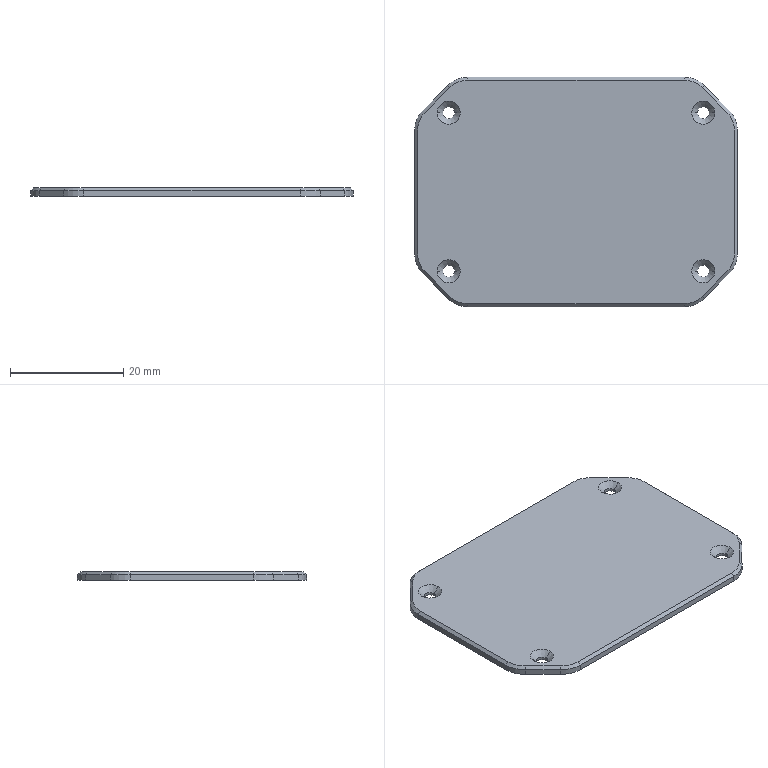NC program | NX | posted with a generic post | part box 57 x 40.5 x 1.5 mm
Lines 4444 to 5919 of 7802:
(PLANAR_PROFILE_COPY_2_COPY_1 , TOOL : D4)
N8676 T01 M6
N8678 G54
N8680 G17 G0 G90 X-121.9 Y151.609 S6500 M3
N8682 G43 Z20. H1
N8684 Z0.1
N8686 G94 G1 Y128.668 Z0.06 F1200.
N8688 X-122.173 Y127.266 Z0.057
N8690 X-122.719 Y125.947 Z0.055
N8692 X-123.518 Y124.763 Z0.052
N8694 X-128.763 Y119.518 Z0.04
N8696 X-129.947 Y118.719 Z0.037
N8698 X-131.266 Y118.173 Z0.035
N8700 X-132.668 Y117.9 Z0.032
N8702 X-172.332 Z-0.037
N8704 X-173.734 Y118.173 Z-0.04
N8706 X-175.053 Y118.719 Z-0.042
N8708 X-176.237 Y119.518 Z-0.045
N8710 X-181.482 Y124.763 Z-0.058
N8712 X-182.281 Y125.947 Z-0.06
N8714 X-182.827 Y127.266 Z-0.063
N8716 X-183.1 Y128.668 Z-0.065
N8718 Y151.832 Z-0.106
N8720 X-182.827 Y153.234 Z-0.108
N8722 X-182.281 Y154.553 Z-0.11
N8724 X-181.482 Y155.737 Z-0.113
N8726 X-176.237 Y160.982 Z-0.126
N8728 X-175.053 Y161.781 Z-0.128
N8730 X-173.734 Y162.327 Z-0.131
N8732 X-172.332 Y162.6 Z-0.133
N8734 X-132.668 Z-0.203
N8736 X-131.266 Y162.327 Z-0.205
N8738 X-129.947 Y161.781 Z-0.208
N8740 X-128.763 Y160.982 Z-0.21
N8742 X-123.518 Y155.737 Z-0.223
N8744 X-122.719 Y154.553 Z-0.226
N8746 X-122.173 Y153.234 Z-0.228
N8748 X-121.9 Y151.832 Z-0.231
N8750 Y128.668 Z-0.271
N8752 X-122.173 Y127.266 Z-0.273
N8754 X-122.719 Y125.947 Z-0.276
N8756 X-123.518 Y124.763 Z-0.278
N8758 X-128.763 Y119.518 Z-0.291
N8760 X-129.947 Y118.719 Z-0.294
N8762 X-131.266 Y118.173 Z-0.296
N8764 X-132.668 Y117.9 Z-0.299
N8766 X-133.321 Z-0.3
N8768 X-171.679 F2000.
N8770 G2 X-176.699 Y119.98 R7.1
N8772 G1 X-181.02 Y124.301
N8774 G2 X-183.1 Y129.321 R7.1
N8776 G1 Y151.179
N8778 G2 X-181.02 Y156.199 R7.1
N8780 G1 X-176.699 Y160.52
N8782 G2 X-171.679 Y162.6 R7.1
N8784 G1 X-133.321
N8786 G2 X-128.301 Y160.52 R7.1
N8788 G1 X-123.98 Y156.199
N8790 G2 X-121.9 Y151.179 R7.1
N8792 G1 Y129.321
N8794 G2 X-123.98 Y124.301 R7.1
N8796 G1 X-128.301 Y119.98
N8798 G2 X-133.321 Y117.9 R7.1
N8800 G1 Z-0.2
N8802 G0 Z20.
N8804 X-121.9 Y151.609
N8806 Z-0.2
N8808 G1 Y128.668 Z-0.24 F1200.
N8810 X-122.173 Y127.266 Z-0.243
N8812 X-122.719 Y125.947 Z-0.245
N8814 X-123.518 Y124.763 Z-0.248
N8816 X-128.763 Y119.518 Z-0.26
N8818 X-129.947 Y118.719 Z-0.263
N8820 X-131.266 Y118.173 Z-0.265
N8822 X-132.668 Y117.9 Z-0.268
N8824 X-172.332 Z-0.337
N8826 X-173.734 Y118.173 Z-0.34
N8828 X-175.053 Y118.719 Z-0.342
N8830 X-176.237 Y119.518 Z-0.345
N8832 X-181.482 Y124.763 Z-0.358
N8834 X-182.281 Y125.947 Z-0.36
N8836 X-182.827 Y127.266 Z-0.363
N8838 X-183.1 Y128.668 Z-0.365
N8840 Y151.832 Z-0.406
N8842 X-182.827 Y153.234 Z-0.408
N8844 X-182.281 Y154.553 Z-0.41
N8846 X-181.482 Y155.737 Z-0.413
N8848 X-176.237 Y160.982 Z-0.426
N8850 X-175.053 Y161.781 Z-0.428
N8852 X-173.734 Y162.327 Z-0.431
N8854 X-172.332 Y162.6 Z-0.433
N8856 X-132.668 Z-0.503
N8858 X-131.266 Y162.327 Z-0.505
N8860 X-129.947 Y161.781 Z-0.508
N8862 X-128.763 Y160.982 Z-0.51
N8864 X-123.518 Y155.737 Z-0.523
N8866 X-122.719 Y154.553 Z-0.526
N8868 X-122.173 Y153.234 Z-0.528
N8870 X-121.9 Y151.832 Z-0.531
N8872 Y128.668 Z-0.571
N8874 X-122.173 Y127.266 Z-0.573
N8876 X-122.719 Y125.947 Z-0.576
N8878 X-123.518 Y124.763 Z-0.578
N8880 X-128.763 Y119.518 Z-0.591
N8882 X-129.947 Y118.719 Z-0.594
N8884 X-131.266 Y118.173 Z-0.596
N8886 X-132.668 Y117.9 Z-0.599
N8888 X-133.321 Z-0.6
N8890 X-171.679 F2000.
N8892 G2 X-176.699 Y119.98 R7.1
N8894 G1 X-181.02 Y124.301
N8896 G2 X-183.1 Y129.321 R7.1
N8898 G1 Y151.179
N8900 G2 X-181.02 Y156.199 R7.1
N8902 G1 X-176.699 Y160.52
N8904 G2 X-171.679 Y162.6 R7.1
N8906 G1 X-133.321
N8908 G2 X-128.301 Y160.52 R7.1
N8910 G1 X-123.98 Y156.199
N8912 G2 X-121.9 Y151.179 R7.1
N8914 G1 Y129.321
N8916 G2 X-123.98 Y124.301 R7.1
N8918 G1 X-128.301 Y119.98
N8920 G2 X-133.321 Y117.9 R7.1
N8922 G1 Z-0.5
N8924 G0 Z20.
N8926 X-121.9 Y151.609
N8928 Z-0.5
N8930 G1 Y128.668 Z-0.54 F1200.
N8932 X-122.173 Y127.266 Z-0.543
N8934 X-122.719 Y125.947 Z-0.545
N8936 X-123.518 Y124.763 Z-0.548
N8938 X-128.763 Y119.518 Z-0.56
N8940 X-129.947 Y118.719 Z-0.563
N8942 X-131.266 Y118.173 Z-0.565
N8944 X-132.668 Y117.9 Z-0.568
N8946 X-172.332 Z-0.637
N8948 X-173.734 Y118.173 Z-0.64
N8950 X-175.053 Y118.719 Z-0.642
N8952 X-176.237 Y119.518 Z-0.645
N8954 X-181.482 Y124.763 Z-0.658
N8956 X-182.281 Y125.947 Z-0.66
N8958 X-182.827 Y127.266 Z-0.663
N8960 X-183.1 Y128.668 Z-0.665
N8962 Y151.832 Z-0.706
N8964 X-182.827 Y153.234 Z-0.708
N8966 X-182.281 Y154.553 Z-0.71
N8968 X-181.482 Y155.737 Z-0.713
N8970 X-176.237 Y160.982 Z-0.726
N8972 X-175.053 Y161.781 Z-0.728
N8974 X-173.734 Y162.327 Z-0.731
N8976 X-172.332 Y162.6 Z-0.733
N8978 X-132.668 Z-0.803
N8980 X-131.266 Y162.327 Z-0.805
N8982 X-129.947 Y161.781 Z-0.808
N8984 X-128.763 Y160.982 Z-0.81
N8986 X-123.518 Y155.737 Z-0.823
N8988 X-122.719 Y154.553 Z-0.826
N8990 X-122.173 Y153.234 Z-0.828
N8992 X-121.9 Y151.832 Z-0.831
N8994 Y128.668 Z-0.871
N8996 X-122.173 Y127.266 Z-0.873
N8998 X-122.719 Y125.947 Z-0.876
N9000 X-123.518 Y124.763 Z-0.878
N9002 X-128.763 Y119.518 Z-0.891
N9004 X-129.947 Y118.719 Z-0.894
N9006 X-131.266 Y118.173 Z-0.896
N9008 X-132.668 Y117.9 Z-0.899
N9010 X-133.321 Z-0.9
N9012 X-171.679 F2000.
N9014 G2 X-176.699 Y119.98 R7.1
N9016 G1 X-181.02 Y124.301
N9018 G2 X-183.1 Y129.321 R7.1
N9020 G1 Y151.179
N9022 G2 X-181.02 Y156.199 R7.1
N9024 G1 X-176.699 Y160.52
N9026 G2 X-171.679 Y162.6 R7.1
N9028 G1 X-133.321
N9030 G2 X-128.301 Y160.52 R7.1
N9032 G1 X-123.98 Y156.199
N9034 G2 X-121.9 Y151.179 R7.1
N9036 G1 Y129.321
N9038 G2 X-123.98 Y124.301 R7.1
N9040 G1 X-128.301 Y119.98
N9042 G2 X-133.321 Y117.9 R7.1
N9044 G1 Z-0.8
N9046 G0 Z20.
N9048 X-121.9 Y151.609
N9050 Z-0.8
N9052 G1 Y128.668 Z-0.84 F1200.
N9054 X-122.173 Y127.266 Z-0.843
N9056 X-122.719 Y125.947 Z-0.845
N9058 X-123.518 Y124.763 Z-0.848
N9060 X-128.763 Y119.518 Z-0.86
N9062 X-129.947 Y118.719 Z-0.863
N9064 X-131.266 Y118.173 Z-0.865
N9066 X-132.668 Y117.9 Z-0.868
N9068 X-172.332 Z-0.937
N9070 X-173.734 Y118.173 Z-0.94
N9072 X-175.053 Y118.719 Z-0.942
N9074 X-176.237 Y119.518 Z-0.945
N9076 X-181.482 Y124.763 Z-0.958
N9078 X-182.281 Y125.947 Z-0.96
N9080 X-182.827 Y127.266 Z-0.963
N9082 X-183.1 Y128.668 Z-0.965
N9084 Y151.832 Z-1.006
N9086 X-182.827 Y153.234 Z-1.008
N9088 X-182.281 Y154.553 Z-1.01
N9090 X-181.482 Y155.737 Z-1.013
N9092 X-176.237 Y160.982 Z-1.026
N9094 X-175.053 Y161.781 Z-1.028
N9096 X-173.734 Y162.327 Z-1.031
N9098 X-172.332 Y162.6 Z-1.033
N9100 X-132.668 Z-1.103
N9102 X-131.266 Y162.327 Z-1.105
N9104 X-129.947 Y161.781 Z-1.108
N9106 X-128.763 Y160.982 Z-1.11
N9108 X-123.518 Y155.737 Z-1.123
N9110 X-122.719 Y154.553 Z-1.126
N9112 X-122.173 Y153.234 Z-1.128
N9114 X-121.9 Y151.832 Z-1.131
N9116 Y128.668 Z-1.171
N9118 X-122.173 Y127.266 Z-1.173
N9120 X-122.719 Y125.947 Z-1.176
N9122 X-123.518 Y124.763 Z-1.178
N9124 X-128.763 Y119.518 Z-1.191
N9126 X-129.947 Y118.719 Z-1.194
N9128 X-131.266 Y118.173 Z-1.196
N9130 X-132.668 Y117.9 Z-1.199
N9132 X-133.321 Z-1.2
N9134 X-171.679 F2000.
N9136 G2 X-176.699 Y119.98 R7.1
N9138 G1 X-181.02 Y124.301
N9140 G2 X-183.1 Y129.321 R7.1
N9142 G1 Y151.179
N9144 G2 X-181.02 Y156.199 R7.1
N9146 G1 X-176.699 Y160.52
N9148 G2 X-171.679 Y162.6 R7.1
N9150 G1 X-133.321
N9152 G2 X-128.301 Y160.52 R7.1
N9154 G1 X-123.98 Y156.199
N9156 G2 X-121.9 Y151.179 R7.1
N9158 G1 Y129.321
N9160 G2 X-123.98 Y124.301 R7.1
N9162 G1 X-128.301 Y119.98
N9164 G2 X-133.321 Y117.9 R7.1
N9166 G1 Z-1.1
N9168 G0 Z20.
N9170 X-121.9 Y151.609
N9172 Z-1.1
N9174 G1 Y128.668 Z-1.14 F1200.
N9176 X-122.173 Y127.266 Z-1.143
N9178 X-122.719 Y125.947 Z-1.145
N9180 X-123.518 Y124.763 Z-1.148
N9182 X-128.763 Y119.518 Z-1.16
N9184 X-129.947 Y118.719 Z-1.163
N9186 X-131.266 Y118.173 Z-1.165
N9188 X-132.668 Y117.9 Z-1.168
N9190 X-172.332 Z-1.237
N9192 X-173.734 Y118.173 Z-1.24
N9194 X-175.053 Y118.719 Z-1.242
N9196 X-176.237 Y119.518 Z-1.245
N9198 X-181.482 Y124.763 Z-1.258
N9200 X-182.281 Y125.947 Z-1.26
N9202 X-182.827 Y127.266 Z-1.263
N9204 X-183.1 Y128.668 Z-1.265
N9206 Y151.832 Z-1.306
N9208 X-182.827 Y153.234 Z-1.308
N9210 X-182.281 Y154.553 Z-1.31
N9212 X-181.482 Y155.737 Z-1.313
N9214 X-176.237 Y160.982 Z-1.326
N9216 X-175.053 Y161.781 Z-1.328
N9218 X-173.734 Y162.327 Z-1.331
N9220 X-172.332 Y162.6 Z-1.333
N9222 X-132.668 Z-1.403
N9224 X-131.266 Y162.327 Z-1.405
N9226 X-129.947 Y161.781 Z-1.408
N9228 X-128.763 Y160.982 Z-1.41
N9230 X-123.518 Y155.737 Z-1.423
N9232 X-122.719 Y154.553 Z-1.426
N9234 X-122.173 Y153.234 Z-1.428
N9236 X-121.9 Y151.832 Z-1.431
N9238 Y128.668 Z-1.471
N9240 X-122.173 Y127.266 Z-1.473
N9242 X-122.719 Y125.947 Z-1.476
N9244 X-123.518 Y124.763 Z-1.478
N9246 X-128.763 Y119.518 Z-1.491
N9248 X-129.947 Y118.719 Z-1.494
N9250 X-131.266 Y118.173 Z-1.496
N9252 X-132.668 Y117.9 Z-1.499
N9254 X-133.321 Z-1.5
N9256 X-171.679 F2000.
N9258 G2 X-176.699 Y119.98 R7.1
N9260 G1 X-181.02 Y124.301
N9262 G2 X-183.1 Y129.321 R7.1
N9264 G1 Y151.179
N9266 G2 X-181.02 Y156.199 R7.1
N9268 G1 X-176.699 Y160.52
N9270 G2 X-171.679 Y162.6 R7.1
N9272 G1 X-133.321
N9274 G2 X-128.301 Y160.52 R7.1
N9276 G1 X-123.98 Y156.199
N9278 G2 X-121.9 Y151.179 R7.1
N9280 G1 Y129.321
N9282 G2 X-123.98 Y124.301 R7.1
N9284 G1 X-128.301 Y119.98
N9286 G2 X-133.321 Y117.9 R7.1
N9288 G1 Z-1.4
N9290 G0 Z20.
(PLANAR_PROFILE_COPY_COPY_2_COPY_1 , TOOL : D4)
N9292 X-133.221
N9294 Z1.5
N9296 G1 Z-1.5 F800.
N9298 X-133.232 Y117.952
N9300 X-133.27 Y117.989
N9302 X-133.321 Y118.
N9304 X-171.679
N9306 G2 X-176.629 Y120.05 R7.
N9308 G1 X-180.95 Y124.371
N9310 G2 X-183. Y129.321 R7.
N9312 G1 Y151.179
N9314 G2 X-180.95 Y156.129 R7.
N9316 G1 X-176.629 Y160.45
N9318 G2 X-171.679 Y162.5 R7.
N9320 G1 X-133.321
N9322 G2 X-128.371 Y160.45 R7.
N9324 G1 X-124.05 Y156.129
N9326 G2 X-122. Y151.179 R7.
N9328 G1 Y129.321
N9330 G2 X-124.05 Y124.371 R7.
N9332 G1 X-128.371 Y120.05
N9334 G2 X-133.321 Y118. R7.
N9336 G1 X-133.373 Y117.989
N9338 X-133.41 Y117.952
N9340 X-133.421 Y117.9
N9342 Z1.5
N9344 G0 Z20.
N9346 M5
(PLANAR_PROFILE_COPY_COPY_COPY_1_COPY_1 , TOOL : D3倒角)
N9348 T02 M6
N9350 G54
N9352 G17 G0 G90 X-131.321 Y117.4 S4500 M3
N9354 G43 Z20. H2
N9356 Z2.
N9358 G94 G1 Z-1. F800.
N9360 G3 X-133.321 Y119.4 R2.
N9362 G1 X-171.679
N9364 G2 X-175.639 Y121.04 R5.6
N9366 G1 X-179.96 Y125.361
N9368 G2 X-181.6 Y129.321 R5.6
N9370 G1 Y151.179
N9372 G2 X-179.96 Y155.139 R5.6
N9374 G1 X-175.639 Y159.46
N9376 G2 X-171.679 Y161.1 R5.6
N9378 G1 X-133.321
N9380 G2 X-129.361 Y159.46 R5.6
N9382 G1 X-125.04 Y155.139
N9384 G2 X-123.4 Y151.179 R5.6
N9386 G1 Y129.321
N9388 G2 X-125.04 Y125.361 R5.6
N9390 G1 X-129.361 Y121.04
N9392 G2 X-133.321 Y119.4 R5.6
N9394 G3 X-135.321 Y117.4 R2.
N9396 G1 Z2.
N9398 G0 Z20.
N9400 M5
(PLANAR_PROFILE_COPY_3_COPY_1 , TOOL : D4)
N9402 T01 M6
N9404 G54
N9406 G17 G0 G90 X-183.9 Y151.609 S6500 M3
N9408 G43 Z20. H1
N9410 Z0.1
N9412 G94 G1 Y128.668 Z0.06 F1200.
N9414 X-184.173 Y127.266 Z0.057
N9416 X-184.719 Y125.947 Z0.055
N9418 X-185.518 Y124.763 Z0.052
N9420 X-190.763 Y119.518 Z0.04
N9422 X-191.947 Y118.719 Z0.037
N9424 X-193.266 Y118.173 Z0.035
N9426 X-194.668 Y117.9 Z0.032
N9428 X-234.332 Z-0.037
N9430 X-235.734 Y118.173 Z-0.04
N9432 X-237.053 Y118.719 Z-0.042
N9434 X-238.237 Y119.518 Z-0.045
N9436 X-243.482 Y124.763 Z-0.058
N9438 X-244.281 Y125.947 Z-0.06
N9440 X-244.827 Y127.266 Z-0.063
N9442 X-245.1 Y128.668 Z-0.065
N9444 Y151.832 Z-0.106
N9446 X-244.827 Y153.234 Z-0.108
N9448 X-244.281 Y154.553 Z-0.11
N9450 X-243.482 Y155.737 Z-0.113
N9452 X-238.237 Y160.982 Z-0.126
N9454 X-237.053 Y161.781 Z-0.128
N9456 X-235.734 Y162.327 Z-0.131
N9458 X-234.332 Y162.6 Z-0.133
N9460 X-194.668 Z-0.203
N9462 X-193.266 Y162.327 Z-0.205
N9464 X-191.947 Y161.781 Z-0.208
N9466 X-190.763 Y160.982 Z-0.21
N9468 X-185.518 Y155.737 Z-0.223
N9470 X-184.719 Y154.553 Z-0.226
N9472 X-184.173 Y153.234 Z-0.228
N9474 X-183.9 Y151.832 Z-0.231
N9476 Y128.668 Z-0.271
N9478 X-184.173 Y127.266 Z-0.273
N9480 X-184.719 Y125.947 Z-0.276
N9482 X-185.518 Y124.763 Z-0.278
N9484 X-190.763 Y119.518 Z-0.291
N9486 X-191.947 Y118.719 Z-0.294
N9488 X-193.266 Y118.173 Z-0.296
N9490 X-194.668 Y117.9 Z-0.299
N9492 X-195.321 Z-0.3
N9494 X-233.679 F2000.
N9496 G2 X-238.699 Y119.98 R7.1
N9498 G1 X-243.02 Y124.301
N9500 G2 X-245.1 Y129.321 R7.1
N9502 G1 Y151.179
N9504 G2 X-243.02 Y156.199 R7.1
N9506 G1 X-238.699 Y160.52
N9508 G2 X-233.679 Y162.6 R7.1
N9510 G1 X-195.321
N9512 G2 X-190.301 Y160.52 R7.1
N9514 G1 X-185.98 Y156.199
N9516 G2 X-183.9 Y151.179 R7.1
N9518 G1 Y129.321
N9520 G2 X-185.98 Y124.301 R7.1
N9522 G1 X-190.301 Y119.98
N9524 G2 X-195.321 Y117.9 R7.1
N9526 G1 Z-0.2
N9528 G0 Z20.
N9530 X-183.9 Y151.609
N9532 Z-0.2
N9534 G1 Y128.668 Z-0.24 F1200.
N9536 X-184.173 Y127.266 Z-0.243
N9538 X-184.719 Y125.947 Z-0.245
N9540 X-185.518 Y124.763 Z-0.248
N9542 X-190.763 Y119.518 Z-0.26
N9544 X-191.947 Y118.719 Z-0.263
N9546 X-193.266 Y118.173 Z-0.265
N9548 X-194.668 Y117.9 Z-0.268
N9550 X-234.332 Z-0.337
N9552 X-235.734 Y118.173 Z-0.34
N9554 X-237.053 Y118.719 Z-0.342
N9556 X-238.237 Y119.518 Z-0.345
N9558 X-243.482 Y124.763 Z-0.358
N9560 X-244.281 Y125.947 Z-0.36
N9562 X-244.827 Y127.266 Z-0.363
N9564 X-245.1 Y128.668 Z-0.365
N9566 Y151.832 Z-0.406
N9568 X-244.827 Y153.234 Z-0.408
N9570 X-244.281 Y154.553 Z-0.41
N9572 X-243.482 Y155.737 Z-0.413
N9574 X-238.237 Y160.982 Z-0.426
N9576 X-237.053 Y161.781 Z-0.428
N9578 X-235.734 Y162.327 Z-0.431
N9580 X-234.332 Y162.6 Z-0.433
N9582 X-194.668 Z-0.503
N9584 X-193.266 Y162.327 Z-0.505
N9586 X-191.947 Y161.781 Z-0.508
N9588 X-190.763 Y160.982 Z-0.51
N9590 X-185.518 Y155.737 Z-0.523
N9592 X-184.719 Y154.553 Z-0.526
N9594 X-184.173 Y153.234 Z-0.528
N9596 X-183.9 Y151.832 Z-0.531
N9598 Y128.668 Z-0.571
N9600 X-184.173 Y127.266 Z-0.573
N9602 X-184.719 Y125.947 Z-0.576
N9604 X-185.518 Y124.763 Z-0.578
N9606 X-190.763 Y119.518 Z-0.591
N9608 X-191.947 Y118.719 Z-0.594
N9610 X-193.266 Y118.173 Z-0.596
N9612 X-194.668 Y117.9 Z-0.599
N9614 X-195.321 Z-0.6
N9616 X-233.679 F2000.
N9618 G2 X-238.699 Y119.98 R7.1
N9620 G1 X-243.02 Y124.301
N9622 G2 X-245.1 Y129.321 R7.1
N9624 G1 Y151.179
N9626 G2 X-243.02 Y156.199 R7.1
N9628 G1 X-238.699 Y160.52
N9630 G2 X-233.679 Y162.6 R7.1
N9632 G1 X-195.321
N9634 G2 X-190.301 Y160.52 R7.1
N9636 G1 X-185.98 Y156.199
N9638 G2 X-183.9 Y151.179 R7.1
N9640 G1 Y129.321
N9642 G2 X-185.98 Y124.301 R7.1
N9644 G1 X-190.301 Y119.98
N9646 G2 X-195.321 Y117.9 R7.1
N9648 G1 Z-0.5
N9650 G0 Z20.
N9652 X-183.9 Y151.609
N9654 Z-0.5
N9656 G1 Y128.668 Z-0.54 F1200.
N9658 X-184.173 Y127.266 Z-0.543
N9660 X-184.719 Y125.947 Z-0.545
N9662 X-185.518 Y124.763 Z-0.548
N9664 X-190.763 Y119.518 Z-0.56
N9666 X-191.947 Y118.719 Z-0.563
N9668 X-193.266 Y118.173 Z-0.565
N9670 X-194.668 Y117.9 Z-0.568
N9672 X-234.332 Z-0.637
N9674 X-235.734 Y118.173 Z-0.64
N9676 X-237.053 Y118.719 Z-0.642
N9678 X-238.237 Y119.518 Z-0.645
N9680 X-243.482 Y124.763 Z-0.658
N9682 X-244.281 Y125.947 Z-0.66
N9684 X-244.827 Y127.266 Z-0.663
N9686 X-245.1 Y128.668 Z-0.665
N9688 Y151.832 Z-0.706
N9690 X-244.827 Y153.234 Z-0.708
N9692 X-244.281 Y154.553 Z-0.71
N9694 X-243.482 Y155.737 Z-0.713
N9696 X-238.237 Y160.982 Z-0.726
N9698 X-237.053 Y161.781 Z-0.728
N9700 X-235.734 Y162.327 Z-0.731
N9702 X-234.332 Y162.6 Z-0.733
N9704 X-194.668 Z-0.803
N9706 X-193.266 Y162.327 Z-0.805
N9708 X-191.947 Y161.781 Z-0.808
N9710 X-190.763 Y160.982 Z-0.81
N9712 X-185.518 Y155.737 Z-0.823
N9714 X-184.719 Y154.553 Z-0.826
N9716 X-184.173 Y153.234 Z-0.828
N9718 X-183.9 Y151.832 Z-0.831
N9720 Y128.668 Z-0.871
N9722 X-184.173 Y127.266 Z-0.873
N9724 X-184.719 Y125.947 Z-0.876
N9726 X-185.518 Y124.763 Z-0.878
N9728 X-190.763 Y119.518 Z-0.891
N9730 X-191.947 Y118.719 Z-0.894
N9732 X-193.266 Y118.173 Z-0.896
N9734 X-194.668 Y117.9 Z-0.899
N9736 X-195.321 Z-0.9
N9738 X-233.679 F2000.
N9740 G2 X-238.699 Y119.98 R7.1
N9742 G1 X-243.02 Y124.301
N9744 G2 X-245.1 Y129.321 R7.1
N9746 G1 Y151.179
N9748 G2 X-243.02 Y156.199 R7.1
N9750 G1 X-238.699 Y160.52
N9752 G2 X-233.679 Y162.6 R7.1
N9754 G1 X-195.321
N9756 G2 X-190.301 Y160.52 R7.1
N9758 G1 X-185.98 Y156.199
N9760 G2 X-183.9 Y151.179 R7.1
N9762 G1 Y129.321
N9764 G2 X-185.98 Y124.301 R7.1
N9766 G1 X-190.301 Y119.98
N9768 G2 X-195.321 Y117.9 R7.1
N9770 G1 Z-0.8
N9772 G0 Z20.
N9774 X-183.9 Y151.609
N9776 Z-0.8
N9778 G1 Y128.668 Z-0.84 F1200.
N9780 X-184.173 Y127.266 Z-0.843
N9782 X-184.719 Y125.947 Z-0.845
N9784 X-185.518 Y124.763 Z-0.848
N9786 X-190.763 Y119.518 Z-0.86
N9788 X-191.947 Y118.719 Z-0.863
N9790 X-193.266 Y118.173 Z-0.865
N9792 X-194.668 Y117.9 Z-0.868
N9794 X-234.332 Z-0.937
N9796 X-235.734 Y118.173 Z-0.94
N9798 X-237.053 Y118.719 Z-0.942
N9800 X-238.237 Y119.518 Z-0.945
N9802 X-243.482 Y124.763 Z-0.958
N9804 X-244.281 Y125.947 Z-0.96
N9806 X-244.827 Y127.266 Z-0.963
N9808 X-245.1 Y128.668 Z-0.965
N9810 Y151.832 Z-1.006
N9812 X-244.827 Y153.234 Z-1.008
N9814 X-244.281 Y154.553 Z-1.01
N9816 X-243.482 Y155.737 Z-1.013
N9818 X-238.237 Y160.982 Z-1.026
N9820 X-237.053 Y161.781 Z-1.028
N9822 X-235.734 Y162.327 Z-1.031
N9824 X-234.332 Y162.6 Z-1.033
N9826 X-194.668 Z-1.103
N9828 X-193.266 Y162.327 Z-1.105
N9830 X-191.947 Y161.781 Z-1.108
N9832 X-190.763 Y160.982 Z-1.11
N9834 X-185.518 Y155.737 Z-1.123
N9836 X-184.719 Y154.553 Z-1.126
N9838 X-184.173 Y153.234 Z-1.128
N9840 X-183.9 Y151.832 Z-1.131
N9842 Y128.668 Z-1.171
N9844 X-184.173 Y127.266 Z-1.173
N9846 X-184.719 Y125.947 Z-1.176
N9848 X-185.518 Y124.763 Z-1.178
N9850 X-190.763 Y119.518 Z-1.191
N9852 X-191.947 Y118.719 Z-1.194
N9854 X-193.266 Y118.173 Z-1.196
N9856 X-194.668 Y117.9 Z-1.199
N9858 X-195.321 Z-1.2
N9860 X-233.679 F2000.
N9862 G2 X-238.699 Y119.98 R7.1
N9864 G1 X-243.02 Y124.301
N9866 G2 X-245.1 Y129.321 R7.1
N9868 G1 Y151.179
N9870 G2 X-243.02 Y156.199 R7.1
N9872 G1 X-238.699 Y160.52
N9874 G2 X-233.679 Y162.6 R7.1
N9876 G1 X-195.321
N9878 G2 X-190.301 Y160.52 R7.1
N9880 G1 X-185.98 Y156.199
N9882 G2 X-183.9 Y151.179 R7.1
N9884 G1 Y129.321
N9886 G2 X-185.98 Y124.301 R7.1
N9888 G1 X-190.301 Y119.98
N9890 G2 X-195.321 Y117.9 R7.1
N9892 G1 Z-1.1
N9894 G0 Z20.
N9896 X-183.9 Y151.609
N9898 Z-1.1
N9900 G1 Y128.668 Z-1.14 F1200.
N9902 X-184.173 Y127.266 Z-1.143
N9904 X-184.719 Y125.947 Z-1.145
N9906 X-185.518 Y124.763 Z-1.148
N9908 X-190.763 Y119.518 Z-1.16
N9910 X-191.947 Y118.719 Z-1.163
N9912 X-193.266 Y118.173 Z-1.165
N9914 X-194.668 Y117.9 Z-1.168
N9916 X-234.332 Z-1.237
N9918 X-235.734 Y118.173 Z-1.24
N9920 X-237.053 Y118.719 Z-1.242
N9922 X-238.237 Y119.518 Z-1.245
N9924 X-243.482 Y124.763 Z-1.258
N9926 X-244.281 Y125.947 Z-1.26
N9928 X-244.827 Y127.266 Z-1.263
N9930 X-245.1 Y128.668 Z-1.265
N9932 Y151.832 Z-1.306
N9934 X-244.827 Y153.234 Z-1.308
N9936 X-244.281 Y154.553 Z-1.31
N9938 X-243.482 Y155.737 Z-1.313
N9940 X-238.237 Y160.982 Z-1.326
N9942 X-237.053 Y161.781 Z-1.328
N9944 X-235.734 Y162.327 Z-1.331
N9946 X-234.332 Y162.6 Z-1.333
N9948 X-194.668 Z-1.403
N9950 X-193.266 Y162.327 Z-1.405
N9952 X-191.947 Y161.781 Z-1.408
N9954 X-190.763 Y160.982 Z-1.41
N9956 X-185.518 Y155.737 Z-1.423
N9958 X-184.719 Y154.553 Z-1.426
N9960 X-184.173 Y153.234 Z-1.428
N9962 X-183.9 Y151.832 Z-1.431
N9964 Y128.668 Z-1.471
N9966 X-184.173 Y127.266 Z-1.473
N9968 X-184.719 Y125.947 Z-1.476
N9970 X-185.518 Y124.763 Z-1.478
N9972 X-190.763 Y119.518 Z-1.491
N9974 X-191.947 Y118.719 Z-1.494
N9976 X-193.266 Y118.173 Z-1.496
N9978 X-194.668 Y117.9 Z-1.499
N9980 X-195.321 Z-1.5
N9982 X-233.679 F2000.
N9984 G2 X-238.699 Y119.98 R7.1
N9986 G1 X-243.02 Y124.301
N9988 G2 X-245.1 Y129.321 R7.1
N9990 G1 Y151.179
N9992 G2 X-243.02 Y156.199 R7.1
N9994 G1 X-238.699 Y160.52
N9996 G2 X-233.679 Y162.6 R7.1
N9998 G1 X-195.321
N10000 G2 X-190.301 Y160.52 R7.1
N10002 G1 X-185.98 Y156.199
N10004 G2 X-183.9 Y151.179 R7.1
N10006 G1 Y129.321
N10008 G2 X-185.98 Y124.301 R7.1
N10010 G1 X-190.301 Y119.98
N10012 G2 X-195.321 Y117.9 R7.1
N10014 G1 Z-1.4
N10016 G0 Z20.
(PLANAR_PROFILE_COPY_COPY_3_COPY_1 , TOOL : D4)
N10018 X-195.221
N10020 Z1.5
N10022 G1 Z-1.5 F800.
N10024 X-195.232 Y117.952
N10026 X-195.27 Y117.989
N10028 X-195.321 Y118.
N10030 X-233.679
N10032 G2 X-238.629 Y120.05 R7.
N10034 G1 X-242.95 Y124.371
N10036 G2 X-245. Y129.321 R7.
N10038 G1 Y151.179
N10040 G2 X-242.95 Y156.129 R7.
N10042 G1 X-238.629 Y160.45
N10044 G2 X-233.679 Y162.5 R7.
N10046 G1 X-195.321
N10048 G2 X-190.371 Y160.45 R7.
N10050 G1 X-186.05 Y156.129
N10052 G2 X-184. Y151.179 R7.
N10054 G1 Y129.321
N10056 G2 X-186.05 Y124.371 R7.
N10058 G1 X-190.371 Y120.05
N10060 G2 X-195.321 Y118. R7.
N10062 G1 X-195.373 Y117.989
N10064 X-195.41 Y117.952
N10066 X-195.421 Y117.9
N10068 Z1.5
N10070 G0 Z20.
N10072 M5
(PLANAR_PROFILE_COPY_COPY_COPY_2_COPY_1 , TOOL : D3倒角)
N10074 T02 M6
N10076 G54
N10078 G17 G0 G90 X-193.321 Y117.4 S4500 M3
N10080 G43 Z20. H2
N10082 Z2.
N10084 G94 G1 Z-1. F800.
N10086 G3 X-195.321 Y119.4 R2.
N10088 G1 X-233.679
N10090 G2 X-237.639 Y121.04 R5.6
N10092 G1 X-241.96 Y125.361
N10094 G2 X-243.6 Y129.321 R5.6
N10096 G1 Y151.179
N10098 G2 X-241.96 Y155.139 R5.6
N10100 G1 X-237.639 Y159.46
N10102 G2 X-233.679 Y161.1 R5.6
N10104 G1 X-195.321
N10106 G2 X-191.361 Y159.46 R5.6
N10108 G1 X-187.04 Y155.139
N10110 G2 X-185.4 Y151.179 R5.6
N10112 G1 Y129.321
N10114 G2 X-187.04 Y125.361 R5.6
N10116 G1 X-191.361 Y121.04
N10118 G2 X-195.321 Y119.4 R5.6
N10120 G3 X-197.321 Y117.4 R2.
N10122 G1 Z2.
N10124 G0 Z20.
N10126 M5
(PLANAR_PROFILE_COPY_4_COPY_1 , TOOL : D4)
N10128 T01 M6
N10130 G54
N10132 G17 G0 G90 X-245.9 Y151.609 S6500 M3
N10134 G43 Z20. H1
N10136 Z0.1
N10138 G94 G1 Y128.668 Z0.06 F1200.
N10140 X-246.173 Y127.266 Z0.057
N10142 X-246.719 Y125.947 Z0.055
N10144 X-247.518 Y124.763 Z0.052
N10146 X-252.763 Y119.518 Z0.04
N10148 X-253.947 Y118.719 Z0.037
N10150 X-255.266 Y118.173 Z0.035
N10152 X-256.668 Y117.9 Z0.032
N10154 X-296.332 Z-0.037
N10156 X-297.734 Y118.173 Z-0.04
N10158 X-299.053 Y118.719 Z-0.042
N10160 X-300.237 Y119.518 Z-0.045
N10162 X-305.482 Y124.763 Z-0.058
N10164 X-306.281 Y125.947 Z-0.06
N10166 X-306.827 Y127.266 Z-0.063
N10168 X-307.1 Y128.668 Z-0.065
N10170 Y151.832 Z-0.106
N10172 X-306.827 Y153.234 Z-0.108
N10174 X-306.281 Y154.553 Z-0.11
N10176 X-305.482 Y155.737 Z-0.113
N10178 X-300.237 Y160.982 Z-0.126
N10180 X-299.053 Y161.781 Z-0.128
N10182 X-297.734 Y162.327 Z-0.131
N10184 X-296.332 Y162.6 Z-0.133
N10186 X-256.668 Z-0.203
N10188 X-255.266 Y162.327 Z-0.205
N10190 X-253.947 Y161.781 Z-0.208
N10192 X-252.763 Y160.982 Z-0.21
N10194 X-247.518 Y155.737 Z-0.223
N10196 X-246.719 Y154.553 Z-0.226
N10198 X-246.173 Y153.234 Z-0.228
N10200 X-245.9 Y151.832 Z-0.231
N10202 Y128.668 Z-0.271
N10204 X-246.173 Y127.266 Z-0.273
N10206 X-246.719 Y125.947 Z-0.276
N10208 X-247.518 Y124.763 Z-0.278
N10210 X-252.763 Y119.518 Z-0.291
N10212 X-253.947 Y118.719 Z-0.294
N10214 X-255.266 Y118.173 Z-0.296
N10216 X-256.668 Y117.9 Z-0.299
N10218 X-257.321 Z-0.3
N10220 X-295.679 F2000.
N10222 G2 X-300.699 Y119.98 R7.1
N10224 G1 X-305.02 Y124.301
N10226 G2 X-307.1 Y129.321 R7.1
N10228 G1 Y151.179
N10230 G2 X-305.02 Y156.199 R7.1
N10232 G1 X-300.699 Y160.52
N10234 G2 X-295.679 Y162.6 R7.1
N10236 G1 X-257.321
N10238 G2 X-252.301 Y160.52 R7.1
N10240 G1 X-247.98 Y156.199
N10242 G2 X-245.9 Y151.179 R7.1
N10244 G1 Y129.321
N10246 G2 X-247.98 Y124.301 R7.1
N10248 G1 X-252.301 Y119.98
N10250 G2 X-257.321 Y117.9 R7.1
N10252 G1 Z-0.2
N10254 G0 Z20.
N10256 X-245.9 Y151.609
N10258 Z-0.2
N10260 G1 Y128.668 Z-0.24 F1200.
N10262 X-246.173 Y127.266 Z-0.243
N10264 X-246.719 Y125.947 Z-0.245
N10266 X-247.518 Y124.763 Z-0.248
N10268 X-252.763 Y119.518 Z-0.26
N10270 X-253.947 Y118.719 Z-0.263
N10272 X-255.266 Y118.173 Z-0.265
N10274 X-256.668 Y117.9 Z-0.268
N10276 X-296.332 Z-0.337
N10278 X-297.734 Y118.173 Z-0.34
N10280 X-299.053 Y118.719 Z-0.342
N10282 X-300.237 Y119.518 Z-0.345
N10284 X-305.482 Y124.763 Z-0.358
N10286 X-306.281 Y125.947 Z-0.36
N10288 X-306.827 Y127.266 Z-0.363
N10290 X-307.1 Y128.668 Z-0.365
N10292 Y151.832 Z-0.406
N10294 X-306.827 Y153.234 Z-0.408
N10296 X-306.281 Y154.553 Z-0.41
N10298 X-305.482 Y155.737 Z-0.413
N10300 X-300.237 Y160.982 Z-0.426
N10302 X-299.053 Y161.781 Z-0.428
N10304 X-297.734 Y162.327 Z-0.431
N10306 X-296.332 Y162.6 Z-0.433
N10308 X-256.668 Z-0.503
N10310 X-255.266 Y162.327 Z-0.505
N10312 X-253.947 Y161.781 Z-0.508
N10314 X-252.763 Y160.982 Z-0.51
N10316 X-247.518 Y155.737 Z-0.523
N10318 X-246.719 Y154.553 Z-0.526
N10320 X-246.173 Y153.234 Z-0.528
N10322 X-245.9 Y151.832 Z-0.531
N10324 Y128.668 Z-0.571
N10326 X-246.173 Y127.266 Z-0.573
N10328 X-246.719 Y125.947 Z-0.576
N10330 X-247.518 Y124.763 Z-0.578
N10332 X-252.763 Y119.518 Z-0.591
N10334 X-253.947 Y118.719 Z-0.594
N10336 X-255.266 Y118.173 Z-0.596
N10338 X-256.668 Y117.9 Z-0.599
N10340 X-257.321 Z-0.6
N10342 X-295.679 F2000.
N10344 G2 X-300.699 Y119.98 R7.1
N10346 G1 X-305.02 Y124.301
N10348 G2 X-307.1 Y129.321 R7.1
N10350 G1 Y151.179
N10352 G2 X-305.02 Y156.199 R7.1
N10354 G1 X-300.699 Y160.52
N10356 G2 X-295.679 Y162.6 R7.1
N10358 G1 X-257.321
N10360 G2 X-252.301 Y160.52 R7.1
N10362 G1 X-247.98 Y156.199
N10364 G2 X-245.9 Y151.179 R7.1
N10366 G1 Y129.321
N10368 G2 X-247.98 Y124.301 R7.1
N10370 G1 X-252.301 Y119.98
N10372 G2 X-257.321 Y117.9 R7.1
N10374 G1 Z-0.5
N10376 G0 Z20.
N10378 X-245.9 Y151.609
N10380 Z-0.5
N10382 G1 Y128.668 Z-0.54 F1200.
N10384 X-246.173 Y127.266 Z-0.543
N10386 X-246.719 Y125.947 Z-0.545
N10388 X-247.518 Y124.763 Z-0.548
N10390 X-252.763 Y119.518 Z-0.56
N10392 X-253.947 Y118.719 Z-0.563
N10394 X-255.266 Y118.173 Z-0.565
N10396 X-256.668 Y117.9 Z-0.568
N10398 X-296.332 Z-0.637
N10400 X-297.734 Y118.173 Z-0.64
N10402 X-299.053 Y118.719 Z-0.642
N10404 X-300.237 Y119.518 Z-0.645
N10406 X-305.482 Y124.763 Z-0.658
N10408 X-306.281 Y125.947 Z-0.66
N10410 X-306.827 Y127.266 Z-0.663
N10412 X-307.1 Y128.668 Z-0.665
N10414 Y151.832 Z-0.706
N10416 X-306.827 Y153.234 Z-0.708
N10418 X-306.281 Y154.553 Z-0.71
N10420 X-305.482 Y155.737 Z-0.713
N10422 X-300.237 Y160.982 Z-0.726
N10424 X-299.053 Y161.781 Z-0.728
N10426 X-297.734 Y162.327 Z-0.731
N10428 X-296.332 Y162.6 Z-0.733
N10430 X-256.668 Z-0.803
N10432 X-255.266 Y162.327 Z-0.805
N10434 X-253.947 Y161.781 Z-0.808
N10436 X-252.763 Y160.982 Z-0.81
N10438 X-247.518 Y155.737 Z-0.823
N10440 X-246.719 Y154.553 Z-0.826
N10442 X-246.173 Y153.234 Z-0.828
N10444 X-245.9 Y151.832 Z-0.831
N10446 Y128.668 Z-0.871
N10448 X-246.173 Y127.266 Z-0.873
N10450 X-246.719 Y125.947 Z-0.876
N10452 X-247.518 Y124.763 Z-0.878
N10454 X-252.763 Y119.518 Z-0.891
N10456 X-253.947 Y118.719 Z-0.894
N10458 X-255.266 Y118.173 Z-0.896
N10460 X-256.668 Y117.9 Z-0.899
N10462 X-257.321 Z-0.9
N10464 X-295.679 F2000.
N10466 G2 X-300.699 Y119.98 R7.1
N10468 G1 X-305.02 Y124.301
N10470 G2 X-307.1 Y129.321 R7.1
N10472 G1 Y151.179
N10474 G2 X-305.02 Y156.199 R7.1
N10476 G1 X-300.699 Y160.52
N10478 G2 X-295.679 Y162.6 R7.1
N10480 G1 X-257.321
N10482 G2 X-252.301 Y160.52 R7.1
N10484 G1 X-247.98 Y156.199
N10486 G2 X-245.9 Y151.179 R7.1
N10488 G1 Y129.321
N10490 G2 X-247.98 Y124.301 R7.1
N10492 G1 X-252.301 Y119.98
N10494 G2 X-257.321 Y117.9 R7.1
N10496 G1 Z-0.8
N10498 G0 Z20.
N10500 X-245.9 Y151.609
N10502 Z-0.8
N10504 G1 Y128.668 Z-0.84 F1200.
N10506 X-246.173 Y127.266 Z-0.843
N10508 X-246.719 Y125.947 Z-0.845
N10510 X-247.518 Y124.763 Z-0.848
N10512 X-252.763 Y119.518 Z-0.86
N10514 X-253.947 Y118.719 Z-0.863
N10516 X-255.266 Y118.173 Z-0.865
N10518 X-256.668 Y117.9 Z-0.868
N10520 X-296.332 Z-0.937
N10522 X-297.734 Y118.173 Z-0.94
N10524 X-299.053 Y118.719 Z-0.942
N10526 X-300.237 Y119.518 Z-0.945
N10528 X-305.482 Y124.763 Z-0.958
N10530 X-306.281 Y125.947 Z-0.96
N10532 X-306.827 Y127.266 Z-0.963
N10534 X-307.1 Y128.668 Z-0.965
N10536 Y151.832 Z-1.006
N10538 X-306.827 Y153.234 Z-1.008
N10540 X-306.281 Y154.553 Z-1.01
N10542 X-305.482 Y155.737 Z-1.013
N10544 X-300.237 Y160.982 Z-1.026
N10546 X-299.053 Y161.781 Z-1.028
N10548 X-297.734 Y162.327 Z-1.031
N10550 X-296.332 Y162.6 Z-1.033
N10552 X-256.668 Z-1.103
N10554 X-255.266 Y162.327 Z-1.105
N10556 X-253.947 Y161.781 Z-1.108
N10558 X-252.763 Y160.982 Z-1.11
N10560 X-247.518 Y155.737 Z-1.123
N10562 X-246.719 Y154.553 Z-1.126
N10564 X-246.173 Y153.234 Z-1.128
N10566 X-245.9 Y151.832 Z-1.131
N10568 Y128.668 Z-1.171
N10570 X-246.173 Y127.266 Z-1.173
N10572 X-246.719 Y125.947 Z-1.176
N10574 X-247.518 Y124.763 Z-1.178
N10576 X-252.763 Y119.518 Z-1.191
N10578 X-253.947 Y118.719 Z-1.194
N10580 X-255.266 Y118.173 Z-1.196
N10582 X-256.668 Y117.9 Z-1.199
N10584 X-257.321 Z-1.2
N10586 X-295.679 F2000.
N10588 G2 X-300.699 Y119.98 R7.1
N10590 G1 X-305.02 Y124.301
N10592 G2 X-307.1 Y129.321 R7.1
N10594 G1 Y151.179
N10596 G2 X-305.02 Y156.199 R7.1
N10598 G1 X-300.699 Y160.52
N10600 G2 X-295.679 Y162.6 R7.1
N10602 G1 X-257.321
N10604 G2 X-252.301 Y160.52 R7.1
N10606 G1 X-247.98 Y156.199
N10608 G2 X-245.9 Y151.179 R7.1
N10610 G1 Y129.321
N10612 G2 X-247.98 Y124.301 R7.1
N10614 G1 X-252.301 Y119.98
N10616 G2 X-257.321 Y117.9 R7.1
N10618 G1 Z-1.1
N10620 G0 Z20.
N10622 X-302.406 Y121.686
N10624 Z-1.1
N10626 G1 X-305.482 Y124.763 Z-1.108 F1200.
N10628 X-306.281 Y125.947 Z-1.11
N10630 X-306.827 Y127.266 Z-1.113
N10632 X-307.1 Y128.668 Z-1.115
N10634 Y151.832 Z-1.156
N10636 X-306.827 Y153.234 Z-1.158
N10638 X-306.281 Y154.553 Z-1.16
N10640 X-305.482 Y155.737 Z-1.163
N10642 X-300.237 Y160.982 Z-1.176
N10644 X-299.053 Y161.781 Z-1.178
N10646 X-297.734 Y162.327 Z-1.181
N10648 X-296.332 Y162.6 Z-1.183
N10650 X-256.668 Z-1.253
N10652 X-255.266 Y162.327 Z-1.255
N10654 X-253.947 Y161.781 Z-1.258
N10656 X-252.763 Y160.982 Z-1.26
N10658 X-247.518 Y155.737 Z-1.273
N10660 X-246.719 Y154.553 Z-1.276
N10662 X-246.173 Y153.234 Z-1.278
N10664 X-245.9 Y151.832 Z-1.281
N10666 Y128.668 Z-1.321
N10668 X-246.173 Y127.266 Z-1.323
N10670 X-246.719 Y125.947 Z-1.326
N10672 X-247.518 Y124.763 Z-1.328
N10674 X-252.763 Y119.518 Z-1.341
N10676 X-253.947 Y118.719 Z-1.344
N10678 X-255.266 Y118.173 Z-1.346
N10680 X-256.668 Y117.9 Z-1.349
N10682 X-257.321 Z-1.35
N10684 X-295.679 F2000.
N10686 G2 X-300.699 Y119.98 R7.1
N10688 G1 X-305.02 Y124.301
N10690 G2 X-307.1 Y129.321 R7.1
N10692 G1 Y151.179
N10694 G2 X-305.02 Y156.199 R7.1
N10696 G1 X-300.699 Y160.52
N10698 G2 X-295.679 Y162.6 R7.1
N10700 G1 X-257.321
N10702 G2 X-252.301 Y160.52 R7.1
N10704 G1 X-247.98 Y156.199
N10706 G2 X-245.9 Y151.179 R7.1
N10708 G1 Y129.321
N10710 G2 X-247.98 Y124.301 R7.1
N10712 G1 X-252.301 Y119.98
N10714 G2 X-257.321 Y117.9 R7.1
N10716 G1 Z-1.25
N10718 G0 Z20.
(PLANAR_PROFILE_COPY_COPY_4_COPY_1 , TOOL : D4)
N10720 X-257.221
N10722 Z1.65
N10724 G1 Z-1.35 F800.
N10726 X-257.232 Y117.952
N10728 X-257.27 Y117.989
N10730 X-257.321 Y118.
N10732 X-295.679
N10734 G2 X-300.629 Y120.05 R7.
N10736 G1 X-304.95 Y124.371
N10738 G2 X-307. Y129.321 R7.
N10740 G1 Y151.179
N10742 G2 X-304.95 Y156.129 R7.
N10744 G1 X-300.629 Y160.45
N10746 G2 X-295.679 Y162.5 R7.
N10748 G1 X-257.321
N10750 G2 X-252.371 Y160.45 R7.
N10752 G1 X-248.05 Y156.129
N10754 G2 X-246. Y151.179 R7.
N10756 G1 Y129.321
N10758 G2 X-248.05 Y124.371 R7.
N10760 G1 X-252.371 Y120.05
N10762 G2 X-257.321 Y118. R7.
N10764 G1 X-257.373 Y117.989
N10766 X-257.41 Y117.952
N10768 X-257.421 Y117.9
N10770 Z1.65
N10772 G0 Z20.
N10774 M5
(PLANAR_PROFILE_COPY_COPY_COPY_3_COPY_1 , TOOL : D3倒角)
N10776 T02 M6
N10778 G54
N10780 G17 G0 G90 X-255.321 Y117.4 S4500 M3
N10782 G43 Z20. H2
N10784 Z2.
N10786 G94 G1 Z-1. F800.
N10788 G3 X-257.321 Y119.4 R2.
N10790 G1 X-295.679
N10792 G2 X-299.639 Y121.04 R5.6
N10794 G1 X-303.96 Y125.361
N10796 G2 X-305.6 Y129.321 R5.6
N10798 G1 Y151.179
N10800 G2 X-303.96 Y155.139 R5.6
N10802 G1 X-299.639 Y159.46
N10804 G2 X-295.679 Y161.1 R5.6
N10806 G1 X-257.321
N10808 G2 X-253.361 Y159.46 R5.6
N10810 G1 X-249.04 Y155.139
N10812 G2 X-247.4 Y151.179 R5.6
N10814 G1 Y129.321
N10816 G2 X-249.04 Y125.361 R5.6
N10818 G1 X-253.361 Y121.04
N10820 G2 X-257.321 Y119.4 R5.6
N10822 G3 X-259.321 Y117.4 R2.
N10824 G1 Z2.
N10826 G0 Z20.
N10828 M5
(PLANAR_PROFILE_COPY_7 , TOOL : D4)
N10830 T01 M6
N10832 G54
N10834 G17 G0 G90 X2.1 Y201.609 S6500 M3
N10836 G43 Z20. H1
N10838 Z0.1
N10840 G94 G1 Y178.668 Z0.06 F1200.
N10842 X1.827 Y177.266 Z0.057
N10844 X1.281 Y175.947 Z0.055
N10846 X0.482 Y174.763 Z0.052
N10848 X-4.763 Y169.518 Z0.04
N10850 X-5.947 Y168.719 Z0.037
N10852 X-7.266 Y168.173 Z0.035
N10854 X-8.668 Y167.9 Z0.032
N10856 X-48.332 Z-0.037
N10858 X-49.734 Y168.173 Z-0.04
N10860 X-51.053 Y168.719 Z-0.042
N10862 X-52.237 Y169.518 Z-0.045
N10864 X-57.482 Y174.763 Z-0.058
N10866 X-58.281 Y175.947 Z-0.06
N10868 X-58.827 Y177.266 Z-0.063
N10870 X-59.1 Y178.668 Z-0.065
N10872 Y201.832 Z-0.106
N10874 X-58.827 Y203.234 Z-0.108
N10876 X-58.281 Y204.553 Z-0.11
N10878 X-57.482 Y205.737 Z-0.113
N10880 X-52.237 Y210.982 Z-0.126
N10882 X-51.053 Y211.781 Z-0.128
N10884 X-49.734 Y212.327 Z-0.131
N10886 X-48.332 Y212.6 Z-0.133
N10888 X-8.668 Z-0.203
N10890 X-7.266 Y212.327 Z-0.205
N10892 X-5.947 Y211.781 Z-0.208
N10894 X-4.763 Y210.982 Z-0.21
N10896 X0.482 Y205.737 Z-0.223
N10898 X1.281 Y204.553 Z-0.226
N10900 X1.827 Y203.234 Z-0.228
N10902 X2.1 Y201.832 Z-0.231
N10904 Y178.668 Z-0.271
N10906 X1.827 Y177.266 Z-0.273
N10908 X1.281 Y175.947 Z-0.276
N10910 X0.482 Y174.763 Z-0.278
N10912 X-4.763 Y169.518 Z-0.291
N10914 X-5.947 Y168.719 Z-0.294
N10916 X-7.266 Y168.173 Z-0.296
N10918 X-8.668 Y167.9 Z-0.299
N10920 X-9.321 Z-0.3
N10922 X-47.679 F2000.
N10924 G2 X-52.699 Y169.98 R7.1
N10926 G1 X-57.02 Y174.301
N10928 G2 X-59.1 Y179.321 R7.1
N10930 G1 Y201.179
N10932 G2 X-57.02 Y206.199 R7.1
N10934 G1 X-52.699 Y210.52
N10936 G2 X-47.679 Y212.6 R7.1
N10938 G1 X-9.321
N10940 G2 X-4.301 Y210.52 R7.1
N10942 G1 X0.02 Y206.199
N10944 G2 X2.1 Y201.179 R7.1
N10946 G1 Y179.321
N10948 G2 X0.02 Y174.301 R7.1
N10950 G1 X-4.301 Y169.98
N10952 G2 X-9.321 Y167.9 R7.1
N10954 G1 Z-0.2
N10956 G0 Z20.
N10958 X2.1 Y201.609
N10960 Z-0.2
N10962 G1 Y178.668 Z-0.24 F1200.
N10964 X1.827 Y177.266 Z-0.243
N10966 X1.281 Y175.947 Z-0.245
N10968 X0.482 Y174.763 Z-0.248
N10970 X-4.763 Y169.518 Z-0.26
N10972 X-5.947 Y168.719 Z-0.263
N10974 X-7.266 Y168.173 Z-0.265
N10976 X-8.668 Y167.9 Z-0.268
N10978 X-48.332 Z-0.337
N10980 X-49.734 Y168.173 Z-0.34
N10982 X-51.053 Y168.719 Z-0.342
N10984 X-52.237 Y169.518 Z-0.345
N10986 X-57.482 Y174.763 Z-0.358
N10988 X-58.281 Y175.947 Z-0.36
N10990 X-58.827 Y177.266 Z-0.363
N10992 X-59.1 Y178.668 Z-0.365
N10994 Y201.832 Z-0.406
N10996 X-58.827 Y203.234 Z-0.408
N10998 X-58.281 Y204.553 Z-0.41
N11000 X-57.482 Y205.737 Z-0.413
N11002 X-52.237 Y210.982 Z-0.426
N11004 X-51.053 Y211.781 Z-0.428
N11006 X-49.734 Y212.327 Z-0.431
N11008 X-48.332 Y212.6 Z-0.433
N11010 X-8.668 Z-0.503
N11012 X-7.266 Y212.327 Z-0.505
N11014 X-5.947 Y211.781 Z-0.508
N11016 X-4.763 Y210.982 Z-0.51
N11018 X0.482 Y205.737 Z-0.523
N11020 X1.281 Y204.553 Z-0.526
N11022 X1.827 Y203.234 Z-0.528
N11024 X2.1 Y201.832 Z-0.531
N11026 Y178.668 Z-0.571
N11028 X1.827 Y177.266 Z-0.573
N11030 X1.281 Y175.947 Z-0.576
N11032 X0.482 Y174.763 Z-0.578
N11034 X-4.763 Y169.518 Z-0.591
N11036 X-5.947 Y168.719 Z-0.594
N11038 X-7.266 Y168.173 Z-0.596
N11040 X-8.668 Y167.9 Z-0.599
N11042 X-9.321 Z-0.6
N11044 X-47.679 F2000.
N11046 G2 X-52.699 Y169.98 R7.1
N11048 G1 X-57.02 Y174.301
N11050 G2 X-59.1 Y179.321 R7.1
N11052 G1 Y201.179
N11054 G2 X-57.02 Y206.199 R7.1
N11056 G1 X-52.699 Y210.52
N11058 G2 X-47.679 Y212.6 R7.1
N11060 G1 X-9.321
N11062 G2 X-4.301 Y210.52 R7.1
N11064 G1 X0.02 Y206.199
N11066 G2 X2.1 Y201.179 R7.1
N11068 G1 Y179.321
N11070 G2 X0.02 Y174.301 R7.1
N11072 G1 X-4.301 Y169.98
N11074 G2 X-9.321 Y167.9 R7.1
N11076 G1 Z-0.5
N11078 G0 Z20.
N11080 X2.1 Y201.609
N11082 Z-0.5
N11084 G1 Y178.668 Z-0.54 F1200.
N11086 X1.827 Y177.266 Z-0.543
N11088 X1.281 Y175.947 Z-0.545
N11090 X0.482 Y174.763 Z-0.548
N11092 X-4.763 Y169.518 Z-0.56
N11094 X-5.947 Y168.719 Z-0.563
N11096 X-7.266 Y168.173 Z-0.565
N11098 X-8.668 Y167.9 Z-0.568
N11100 X-48.332 Z-0.637
N11102 X-49.734 Y168.173 Z-0.64
N11104 X-51.053 Y168.719 Z-0.642
N11106 X-52.237 Y169.518 Z-0.645
N11108 X-57.482 Y174.763 Z-0.658
N11110 X-58.281 Y175.947 Z-0.66
N11112 X-58.827 Y177.266 Z-0.663
N11114 X-59.1 Y178.668 Z-0.665
N11116 Y201.832 Z-0.706
N11118 X-58.827 Y203.234 Z-0.708
N11120 X-58.281 Y204.553 Z-0.71
N11122 X-57.482 Y205.737 Z-0.713
N11124 X-52.237 Y210.982 Z-0.726
N11126 X-51.053 Y211.781 Z-0.728
N11128 X-49.734 Y212.327 Z-0.731
N11130 X-48.332 Y212.6 Z-0.733
N11132 X-8.668 Z-0.803
N11134 X-7.266 Y212.327 Z-0.805
N11136 X-5.947 Y211.781 Z-0.808
N11138 X-4.763 Y210.982 Z-0.81
N11140 X0.482 Y205.737 Z-0.823
N11142 X1.281 Y204.553 Z-0.826
N11144 X1.827 Y203.234 Z-0.828
N11146 X2.1 Y201.832 Z-0.831
N11148 Y178.668 Z-0.871
N11150 X1.827 Y177.266 Z-0.873
N11152 X1.281 Y175.947 Z-0.876
N11154 X0.482 Y174.763 Z-0.878
N11156 X-4.763 Y169.518 Z-0.891
N11158 X-5.947 Y168.719 Z-0.894
N11160 X-7.266 Y168.173 Z-0.896
N11162 X-8.668 Y167.9 Z-0.899
N11164 X-9.321 Z-0.9
N11166 X-47.679 F2000.
N11168 G2 X-52.699 Y169.98 R7.1
N11170 G1 X-57.02 Y174.301
N11172 G2 X-59.1 Y179.321 R7.1
N11174 G1 Y201.179
N11176 G2 X-57.02 Y206.199 R7.1
N11178 G1 X-52.699 Y210.52
N11180 G2 X-47.679 Y212.6 R7.1
N11182 G1 X-9.321
N11184 G2 X-4.301 Y210.52 R7.1
N11186 G1 X0.02 Y206.199
N11188 G2 X2.1 Y201.179 R7.1
N11190 G1 Y179.321
N11192 G2 X0.02 Y174.301 R7.1
N11194 G1 X-4.301 Y169.98
N11196 G2 X-9.321 Y167.9 R7.1
N11198 G1 Z-0.8
N11200 G0 Z20.
N11202 X2.1 Y201.609
N11204 Z-0.8
N11206 G1 Y178.668 Z-0.84 F1200.
N11208 X1.827 Y177.266 Z-0.843
N11210 X1.281 Y175.947 Z-0.845
N11212 X0.482 Y174.763 Z-0.848
N11214 X-4.763 Y169.518 Z-0.86
N11216 X-5.947 Y168.719 Z-0.863
N11218 X-7.266 Y168.173 Z-0.865
N11220 X-8.668 Y167.9 Z-0.868
N11222 X-48.332 Z-0.937
N11224 X-49.734 Y168.173 Z-0.94
N11226 X-51.053 Y168.719 Z-0.942
N11228 X-52.237 Y169.518 Z-0.945
N11230 X-57.482 Y174.763 Z-0.958
N11232 X-58.281 Y175.947 Z-0.96
N11234 X-58.827 Y177.266 Z-0.963
N11236 X-59.1 Y178.668 Z-0.965
N11238 Y201.832 Z-1.006
N11240 X-58.827 Y203.234 Z-1.008
N11242 X-58.281 Y204.553 Z-1.01
N11244 X-57.482 Y205.737 Z-1.013
N11246 X-52.237 Y210.982 Z-1.026
N11248 X-51.053 Y211.781 Z-1.028
N11250 X-49.734 Y212.327 Z-1.031
N11252 X-48.332 Y212.6 Z-1.033
N11254 X-8.668 Z-1.103
N11256 X-7.266 Y212.327 Z-1.105
N11258 X-5.947 Y211.781 Z-1.108
N11260 X-4.763 Y210.982 Z-1.11
N11262 X0.482 Y205.737 Z-1.123
N11264 X1.281 Y204.553 Z-1.126
N11266 X1.827 Y203.234 Z-1.128
N11268 X2.1 Y201.832 Z-1.131
N11270 Y178.668 Z-1.171
N11272 X1.827 Y177.266 Z-1.173
N11274 X1.281 Y175.947 Z-1.176
N11276 X0.482 Y174.763 Z-1.178
N11278 X-4.763 Y169.518 Z-1.191
N11280 X-5.947 Y168.719 Z-1.194
N11282 X-7.266 Y168.173 Z-1.196
N11284 X-8.668 Y167.9 Z-1.199
N11286 X-9.321 Z-1.2
N11288 X-47.679 F2000.
N11290 G2 X-52.699 Y169.98 R7.1
N11292 G1 X-57.02 Y174.301
N11294 G2 X-59.1 Y179.321 R7.1
N11296 G1 Y201.179
N11298 G2 X-57.02 Y206.199 R7.1
N11300 G1 X-52.699 Y210.52
N11302 G2 X-47.679 Y212.6 R7.1
N11304 G1 X-9.321
N11306 G2 X-4.301 Y210.52 R7.1
N11308 G1 X0.02 Y206.199
N11310 G2 X2.1 Y201.179 R7.1
N11312 G1 Y179.321
N11314 G2 X0.02 Y174.301 R7.1
N11316 G1 X-4.301 Y169.98
N11318 G2 X-9.321 Y167.9 R7.1
N11320 G1 Z-1.1
N11322 G0 Z20.
N11324 X2.1 Y201.609
N11326 Z-1.1
N11328 G1 Y178.668 Z-1.14 F1200.
N11330 X1.827 Y177.266 Z-1.143
N11332 X1.281 Y175.947 Z-1.145
N11334 X0.482 Y174.763 Z-1.148
N11336 X-4.763 Y169.518 Z-1.16
N11338 X-5.947 Y168.719 Z-1.163
N11340 X-7.266 Y168.173 Z-1.165
N11342 X-8.668 Y167.9 Z-1.168
N11344 X-48.332 Z-1.237
N11346 X-49.734 Y168.173 Z-1.24
N11348 X-51.053 Y168.719 Z-1.242
N11350 X-52.237 Y169.518 Z-1.245
N11352 X-57.482 Y174.763 Z-1.258
N11354 X-58.281 Y175.947 Z-1.26
N11356 X-58.827 Y177.266 Z-1.263
N11358 X-59.1 Y178.668 Z-1.265
N11360 Y201.832 Z-1.306
N11362 X-58.827 Y203.234 Z-1.308
N11364 X-58.281 Y204.553 Z-1.31
N11366 X-57.482 Y205.737 Z-1.313
N11368 X-52.237 Y210.982 Z-1.326
N11370 X-51.053 Y211.781 Z-1.328
N11372 X-49.734 Y212.327 Z-1.331
N11374 X-48.332 Y212.6 Z-1.333
N11376 X-8.668 Z-1.403
N11378 X-7.266 Y212.327 Z-1.405
N11380 X-5.947 Y211.781 Z-1.408
N11382 X-4.763 Y210.982 Z-1.41
N11384 X0.482 Y205.737 Z-1.423
N11386 X1.281 Y204.553 Z-1.426
N11388 X1.827 Y203.234 Z-1.428
N11390 X2.1 Y201.832 Z-1.431
N11392 Y178.668 Z-1.471
N11394 X1.827 Y177.266 Z-1.473
N11396 X1.281 Y175.947 Z-1.476
N11398 X0.482 Y174.763 Z-1.478
N11400 X-4.763 Y169.518 Z-1.491
N11402 X-5.947 Y168.719 Z-1.494
N11404 X-7.266 Y168.173 Z-1.496
N11406 X-8.668 Y167.9 Z-1.499
N11408 X-9.321 Z-1.5
N11410 X-47.679 F2000.
N11412 G2 X-52.699 Y169.98 R7.1
N11414 G1 X-57.02 Y174.301
N11416 G2 X-59.1 Y179.321 R7.1
N11418 G1 Y201.179
N11420 G2 X-57.02 Y206.199 R7.1
N11422 G1 X-52.699 Y210.52
N11424 G2 X-47.679 Y212.6 R7.1
N11426 G1 X-9.321
N11428 G2 X-4.301 Y210.52 R7.1
N11430 G1 X0.02 Y206.199
N11432 G2 X2.1 Y201.179 R7.1
N11434 G1 Y179.321
N11436 G2 X0.02 Y174.301 R7.1
N11438 G1 X-4.301 Y169.98
N11440 G2 X-9.321 Y167.9 R7.1
N11442 G1 Z-1.4
N11444 G0 Z20.
(PLANAR_PROFILE_COPY_COPY_7 , TOOL : D4)
N11446 X-9.221
N11448 Z1.5
N11450 G1 Z-1.5 F800.
N11452 X-9.232 Y167.952
N11454 X-9.27 Y167.989
N11456 X-9.321 Y168.
N11458 X-47.679
N11460 G2 X-52.629 Y170.05 R7.
N11462 G1 X-56.95 Y174.371
N11464 G2 X-59. Y179.321 R7.
N11466 G1 Y201.179
N11468 G2 X-56.95 Y206.129 R7.
N11470 G1 X-52.629 Y210.45
N11472 G2 X-47.679 Y212.5 R7.
N11474 G1 X-9.321
N11476 G2 X-4.371 Y210.45 R7.
N11478 G1 X-0.05 Y206.129
N11480 G2 X2. Y201.179 R7.
N11482 G1 Y179.321
N11484 G2 X-0.05 Y174.371 R7.
N11486 G1 X-4.371 Y170.05
N11488 G2 X-9.321 Y168. R7.
N11490 G1 X-9.373 Y167.989
N11492 X-9.41 Y167.952
N11494 X-9.421 Y167.9
N11496 Z1.5
N11498 G0 Z20.
N11500 M5
(PLANAR_PROFILE_COPY_COPY_COPY_6 , TOOL : D3倒角)
N11502 T02 M6
N11504 G54
N11506 G17 G0 G90 X-7.321 Y167.4 S4500 M3
N11508 G43 Z20. H2
N11510 Z2.
N11512 G94 G1 Z-1. F800.
N11514 G3 X-9.321 Y169.4 R2.
N11516 G1 X-47.679
N11518 G2 X-51.639 Y171.04 R5.6
N11520 G1 X-55.96 Y175.361
N11522 G2 X-57.6 Y179.321 R5.6
N11524 G1 Y201.179
N11526 G2 X-55.96 Y205.139 R5.6
N11528 G1 X-51.639 Y209.46
N11530 G2 X-47.679 Y211.1 R5.6
N11532 G1 X-9.321
N11534 G2 X-5.361 Y209.46 R5.6
N11536 G1 X-1.04 Y205.139
N11538 G2 X0.6 Y201.179 R5.6
N11540 G1 Y179.321
N11542 G2 X-1.04 Y175.361 R5.6
N11544 G1 X-5.361 Y171.04
N11546 G2 X-9.321 Y169.4 R5.6
N11548 G3 X-11.321 Y167.4 R2.
N11550 G1 Z2.
N11552 G0 Z20.
N11554 M5